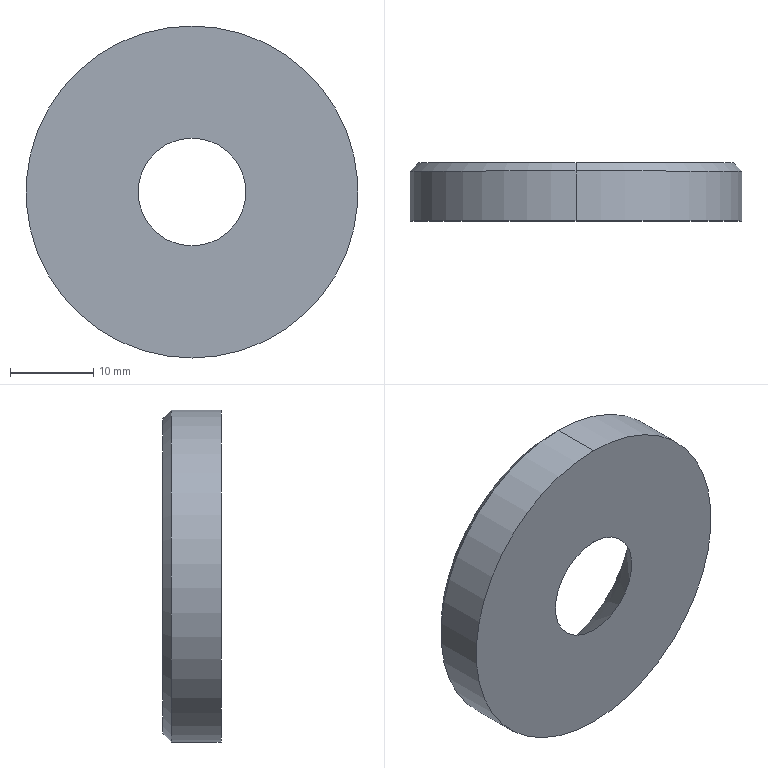Part | SolidWorks | features MBimport 1 | 1 solid | 8 faces | box 40 x 7 x 40 mm | volume 6446 mm3 | cone 4 | plane 2 | cylinder 2 | commonest cylinder face diameters 40 x2
STEP:
#1=CARTESIAN_POINT('',(0.,14.875,6.5));
#2=VERTEX_POINT('',#1);
#3=CARTESIAN_POINT('',(0.,14.875,-6.5));
#4=VERTEX_POINT('',#3);
#5=CARTESIAN_POINT('',(0.,14.875,0.));
#6=DIRECTION('',(0.,-1.,0.));
#7=DIRECTION('',(0.,0.,-1.));
#8=AXIS2_PLACEMENT_3D('',#5,#6,#7);
#9=CIRCLE('',#8,6.5);
#10=EDGE_CURVE('',#2,#4,#9,.T.);
#11=ORIENTED_EDGE('',*,*,#10,.F.);
#12=CARTESIAN_POINT('',(0.,14.875,0.));
#13=DIRECTION('',(0.,-1.,0.));
#14=DIRECTION('',(0.,0.,-1.));
#15=AXIS2_PLACEMENT_3D('',#12,#13,#14);
#16=CIRCLE('',#15,6.5);
#17=EDGE_CURVE('',#4,#2,#16,.T.);
#18=ORIENTED_EDGE('',*,*,#17,.F.);
#19=EDGE_LOOP('',(#11,#18));
#20=FACE_BOUND('',#19,.T.);
#21=CARTESIAN_POINT('',(0.,14.875,-20.));
#22=VERTEX_POINT('',#21);
#23=CARTESIAN_POINT('',(0.,14.875,20.));
#24=VERTEX_POINT('',#23);
#25=CARTESIAN_POINT('',(0.,14.875,0.));
#26=DIRECTION('',(0.,-1.,0.));
#27=DIRECTION('',(0.,0.,-1.));
#28=AXIS2_PLACEMENT_3D('',#25,#26,#27);
#29=CIRCLE('',#28,20.);
#30=EDGE_CURVE('',#22,#24,#29,.T.);
#31=ORIENTED_EDGE('',*,*,#30,.T.);
#32=CARTESIAN_POINT('',(0.,14.875,0.));
#33=DIRECTION('',(0.,-1.,0.));
#34=DIRECTION('',(0.,0.,-1.));
#35=AXIS2_PLACEMENT_3D('',#32,#33,#34);
#36=CIRCLE('',#35,20.);
#37=EDGE_CURVE('',#24,#22,#36,.T.);
#38=ORIENTED_EDGE('',*,*,#37,.T.);
#39=EDGE_LOOP('',(#31,#38));
#40=FACE_OUTER_BOUND('',#39,.T.);
#41=CARTESIAN_POINT('',(-6.5,14.875,0.));
#42=DIRECTION('',(0.,1.,0.));
#43=DIRECTION('',(1.,0.,0.));
#44=AXIS2_PLACEMENT_3D('',#41,#42,#43);
#45=PLANE('',#44);
#46=ADVANCED_FACE('',(#20,#40),#45,.F.);
#47=CARTESIAN_POINT('',(0.,21.875,-13.5));
#48=VERTEX_POINT('',#47);
#49=CARTESIAN_POINT('',(0.,14.875,-6.5));
#50=DIRECTION('',(0.,0.7071,-0.7071));
#51=VECTOR('',#50,1000.);
#52=LINE('',#49,#51);
#53=EDGE_CURVE('',#4,#48,#52,.T.);
#54=ORIENTED_EDGE('',*,*,#53,.F.);
#55=ORIENTED_EDGE('',*,*,#17,.T.);
#56=CARTESIAN_POINT('',(0.,21.875,13.5));
#57=VERTEX_POINT('',#56);
#58=CARTESIAN_POINT('',(0.,14.875,6.5));
#59=DIRECTION('',(0.,0.7071,0.7071));
#60=VECTOR('',#59,1000.);
#61=LINE('',#58,#60);
#62=EDGE_CURVE('',#2,#57,#61,.T.);
#63=ORIENTED_EDGE('',*,*,#62,.T.);
#64=CARTESIAN_POINT('',(0.,21.875,0.));
#65=DIRECTION('',(0.,-1.,0.));
#66=DIRECTION('',(0.,0.,-1.));
#67=AXIS2_PLACEMENT_3D('',#64,#65,#66);
#68=CIRCLE('',#67,13.5);
#69=EDGE_CURVE('',#48,#57,#68,.T.);
#70=ORIENTED_EDGE('',*,*,#69,.F.);
#71=EDGE_LOOP('',(#54,#55,#63,#70));
#72=FACE_OUTER_BOUND('',#71,.T.);
#73=CARTESIAN_POINT('',(0.,14.875,0.));
#74=DIRECTION('',(0.,1.,0.));
#75=DIRECTION('',(0.,0.,1.));
#76=AXIS2_PLACEMENT_3D('',#73,#74,#75);
#77=CONICAL_SURFACE('',#76,6.5,0.7854);
#78=ADVANCED_FACE('',(#72),#77,.F.);
#79=CARTESIAN_POINT('',(0.,21.875,0.));
#80=DIRECTION('',(0.,-1.,0.));
#81=DIRECTION('',(0.,0.,-1.));
#82=AXIS2_PLACEMENT_3D('',#79,#80,#81);
#83=CIRCLE('',#82,13.5);
#84=EDGE_CURVE('',#57,#48,#83,.T.);
#85=ORIENTED_EDGE('',*,*,#84,.T.);
#86=ORIENTED_EDGE('',*,*,#69,.T.);
#87=EDGE_LOOP('',(#85,#86));
#88=FACE_BOUND('',#87,.T.);
#89=CARTESIAN_POINT('',(0.,21.875,-19.));
#90=VERTEX_POINT('',#89);
#91=CARTESIAN_POINT('',(0.,21.875,19.));
#92=VERTEX_POINT('',#91);
#93=CARTESIAN_POINT('',(0.,21.875,0.));
#94=DIRECTION('',(0.,-1.,0.));
#95=DIRECTION('',(0.,0.,-1.));
#96=AXIS2_PLACEMENT_3D('',#93,#94,#95);
#97=CIRCLE('',#96,19.);
#98=EDGE_CURVE('',#90,#92,#97,.T.);
#99=ORIENTED_EDGE('',*,*,#98,.F.);
#100=CARTESIAN_POINT('',(0.,21.875,0.));
#101=DIRECTION('',(0.,-1.,0.));
#102=DIRECTION('',(0.,0.,-1.));
#103=AXIS2_PLACEMENT_3D('',#100,#101,#102);
#104=CIRCLE('',#103,19.);
#105=EDGE_CURVE('',#92,#90,#104,.T.);
#106=ORIENTED_EDGE('',*,*,#105,.F.);
#107=EDGE_LOOP('',(#99,#106));
#108=FACE_OUTER_BOUND('',#107,.T.);
#109=CARTESIAN_POINT('',(-19.,21.875,0.));
#110=DIRECTION('',(0.,-1.,0.));
#111=DIRECTION('',(0.,0.,-1.));
#112=AXIS2_PLACEMENT_3D('',#109,#110,#111);
#113=PLANE('',#112);
#114=ADVANCED_FACE('',(#88,#108),#113,.F.);
#115=CARTESIAN_POINT('',(0.,20.875,20.));
#116=VERTEX_POINT('',#115);
#117=CARTESIAN_POINT('',(0.,21.875,19.));
#118=DIRECTION('',(0.,-0.7071,0.7071));
#119=VECTOR('',#118,1000.);
#120=LINE('',#117,#119);
#121=EDGE_CURVE('',#92,#116,#120,.T.);
#122=ORIENTED_EDGE('',*,*,#121,.F.);
#123=ORIENTED_EDGE('',*,*,#105,.T.);
#124=CARTESIAN_POINT('',(0.,20.875,-20.));
#125=VERTEX_POINT('',#124);
#126=CARTESIAN_POINT('',(0.,21.875,-19.));
#127=DIRECTION('',(0.,-0.7071,-0.7071));
#128=VECTOR('',#127,1000.);
#129=LINE('',#126,#128);
#130=EDGE_CURVE('',#90,#125,#129,.T.);
#131=ORIENTED_EDGE('',*,*,#130,.T.);
#132=CARTESIAN_POINT('',(0.,20.875,0.));
#133=DIRECTION('',(0.,-1.,0.));
#134=DIRECTION('',(0.,0.,-1.));
#135=AXIS2_PLACEMENT_3D('',#132,#133,#134);
#136=CIRCLE('',#135,20.);
#137=EDGE_CURVE('',#116,#125,#136,.T.);
#138=ORIENTED_EDGE('',*,*,#137,.F.);
#139=EDGE_LOOP('',(#122,#123,#131,#138));
#140=FACE_OUTER_BOUND('',#139,.T.);
#141=CARTESIAN_POINT('',(0.,21.875,0.));
#142=DIRECTION('',(0.,-1.,0.));
#143=DIRECTION('',(0.,0.,-1.));
#144=AXIS2_PLACEMENT_3D('',#141,#142,#143);
#145=CONICAL_SURFACE('',#144,19.,0.7854);
#146=ADVANCED_FACE('',(#140),#145,.T.);
#147=CARTESIAN_POINT('',(0.,0.,20.));
#148=DIRECTION('',(0.,-1.,0.));
#149=VECTOR('',#148,1000.);
#150=LINE('',#147,#149);
#151=EDGE_CURVE('',#116,#24,#150,.T.);
#152=ORIENTED_EDGE('',*,*,#151,.F.);
#153=ORIENTED_EDGE('',*,*,#137,.T.);
#154=CARTESIAN_POINT('',(0.,0.,-20.));
#155=DIRECTION('',(0.,-1.,0.));
#156=VECTOR('',#155,1000.);
#157=LINE('',#154,#156);
#158=EDGE_CURVE('',#125,#22,#157,.T.);
#159=ORIENTED_EDGE('',*,*,#158,.T.);
#160=ORIENTED_EDGE('',*,*,#37,.F.);
#161=EDGE_LOOP('',(#152,#153,#159,#160));
#162=FACE_OUTER_BOUND('',#161,.T.);
#163=CARTESIAN_POINT('',(0.,0.,0.));
#164=DIRECTION('',(0.,-1.,0.));
#165=DIRECTION('',(0.,0.,-1.));
#166=AXIS2_PLACEMENT_3D('',#163,#164,#165);
#167=CYLINDRICAL_SURFACE('',#166,20.);
#168=ADVANCED_FACE('',(#162),#167,.T.);
#169=CARTESIAN_POINT('',(0.,20.875,0.));
#170=DIRECTION('',(0.,-1.,0.));
#171=DIRECTION('',(0.,0.,-1.));
#172=AXIS2_PLACEMENT_3D('',#169,#170,#171);
#173=CIRCLE('',#172,20.);
#174=EDGE_CURVE('',#125,#116,#173,.T.);
#175=ORIENTED_EDGE('',*,*,#174,.T.);
#176=ORIENTED_EDGE('',*,*,#151,.T.);
#177=ORIENTED_EDGE('',*,*,#30,.F.);
#178=ORIENTED_EDGE('',*,*,#158,.F.);
#179=EDGE_LOOP('',(#175,#176,#177,#178));
#180=FACE_OUTER_BOUND('',#179,.T.);
#181=CARTESIAN_POINT('',(0.,0.,0.));
#182=DIRECTION('',(0.,-1.,0.));
#183=DIRECTION('',(0.,0.,-1.));
#184=AXIS2_PLACEMENT_3D('',#181,#182,#183);
#185=CYLINDRICAL_SURFACE('',#184,20.);
#186=ADVANCED_FACE('',(#180),#185,.T.);
#187=ORIENTED_EDGE('',*,*,#98,.T.);
#188=ORIENTED_EDGE('',*,*,#121,.T.);
#189=ORIENTED_EDGE('',*,*,#174,.F.);
#190=ORIENTED_EDGE('',*,*,#130,.F.);
#191=EDGE_LOOP('',(#187,#188,#189,#190));
#192=FACE_OUTER_BOUND('',#191,.T.);
#193=CARTESIAN_POINT('',(0.,21.875,0.));
#194=DIRECTION('',(0.,-1.,0.));
#195=DIRECTION('',(0.,0.,-1.));
#196=AXIS2_PLACEMENT_3D('',#193,#194,#195);
#197=CONICAL_SURFACE('',#196,19.,0.7854);
#198=ADVANCED_FACE('',(#192),#197,.T.);
#199=ORIENTED_EDGE('',*,*,#10,.T.);
#200=ORIENTED_EDGE('',*,*,#53,.T.);
#201=ORIENTED_EDGE('',*,*,#84,.F.);
#202=ORIENTED_EDGE('',*,*,#62,.F.);
#203=EDGE_LOOP('',(#199,#200,#201,#202));
#204=FACE_OUTER_BOUND('',#203,.T.);
#205=CARTESIAN_POINT('',(0.,14.875,0.));
#206=DIRECTION('',(0.,1.,0.));
#207=DIRECTION('',(0.,0.,1.));
#208=AXIS2_PLACEMENT_3D('',#205,#206,#207);
#209=CONICAL_SURFACE('',#208,6.5,0.7854);
#210=ADVANCED_FACE('',(#204),#209,.F.);
#211=CLOSED_SHELL('',(#46,#78,#114,#146,#168,#186,#198,#210));
#212=MANIFOLD_SOLID_BREP('',#211);
#213=CARTESIAN_POINT('',(0.,0.,0.));
#214=DIRECTION('',(0.,0.,1.));
#215=DIRECTION('',(1.,0.,0.));
#216=AXIS2_PLACEMENT_3D('',#213,#214,#215);
#217=(LENGTH_UNIT()NAMED_UNIT(*)SI_UNIT(.MILLI.,.METRE.));
#218=UNCERTAINTY_MEASURE_WITH_UNIT(LENGTH_MEASURE(0.00001),#217,'','');
#219=(NAMED_UNIT(*)PLANE_ANGLE_UNIT()SI_UNIT($,.RADIAN.));
#220=(NAMED_UNIT(*)SI_UNIT($,.STERADIAN.)SOLID_ANGLE_UNIT());
#221=(GEOMETRIC_REPRESENTATION_CONTEXT(3)GLOBAL_UNCERTAINTY_ASSIGNED_CONTEXT((#218))GLOBAL_UNIT_ASSIGNED_CONTEXT((#217,#219,#220))REPRESENTATION_CONTEXT('',''));
#222=ADVANCED_BREP_SHAPE_REPRESENTATION('',(#212,#216),#221);